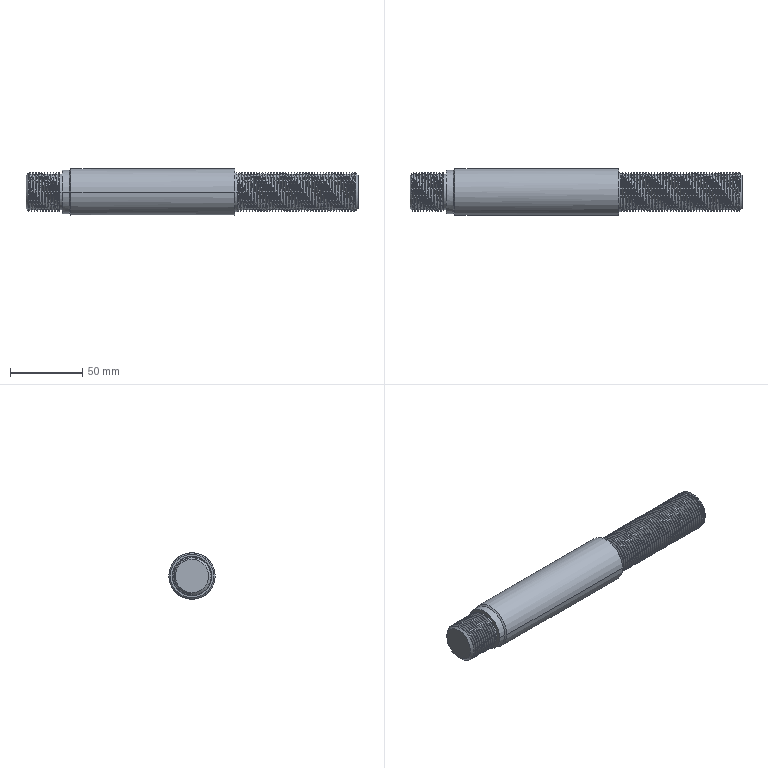Part | SolidWorks | features BaseBody 1 | 1 solid | 134 faces | box 229 x 32 x 32 mm | volume 152492 mm3 | cylinder 111 | plane 9 | cone 8 | spline 6 | commonest cylinder face diameters 27 x105 24.5 x2 30 x2 32 x2